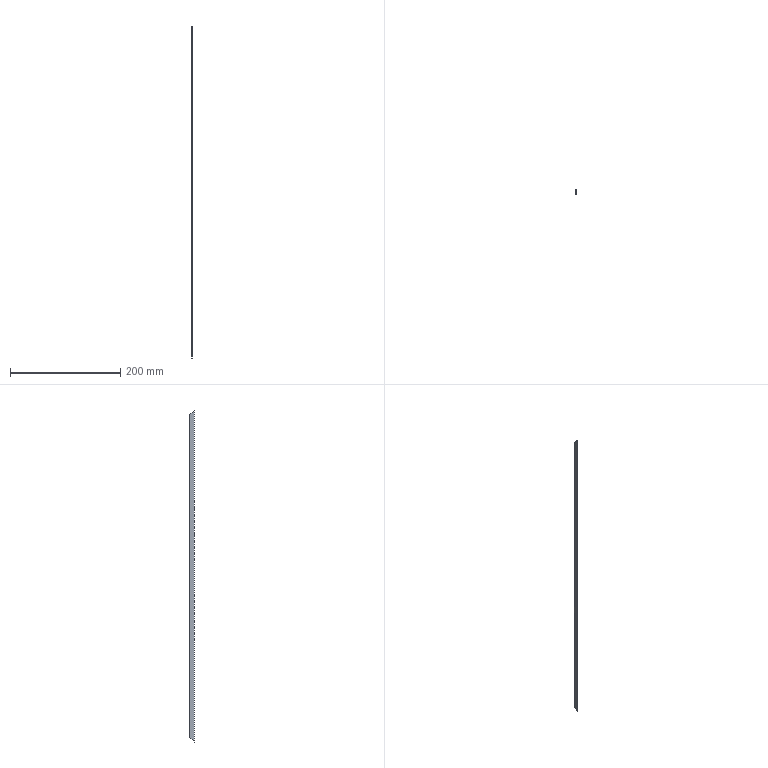Part | NX | features BREP 1 | 1 solid | 6 faces | box 1.5 x 8 x 603 mm | volume 7140 mm3 | plane 6
STEP:
#1=CARTESIAN_POINT('',(0.,8.,293.5));
#2=VERTEX_POINT('',#1);
#3=CARTESIAN_POINT('',(0.,8.,-293.5));
#4=VERTEX_POINT('',#3);
#5=CARTESIAN_POINT('',(0.,8.,301.5));
#6=DIRECTION('',(0.,0.,-1.));
#7=VECTOR('',#6,1000.);
#8=LINE('',#5,#7);
#9=EDGE_CURVE('',#2,#4,#8,.T.);
#10=ORIENTED_EDGE('',*,*,#9,.T.);
#11=CARTESIAN_POINT('',(0.,0.,-301.5));
#12=VERTEX_POINT('',#11);
#13=CARTESIAN_POINT('',(0.,8.,-293.5));
#14=DIRECTION('',(0.,-0.7071,-0.7071));
#15=VECTOR('',#14,1000.);
#16=LINE('',#13,#15);
#17=EDGE_CURVE('',#4,#12,#16,.T.);
#18=ORIENTED_EDGE('',*,*,#17,.T.);
#19=CARTESIAN_POINT('',(0.,0.,301.5));
#20=VERTEX_POINT('',#19);
#21=CARTESIAN_POINT('',(0.,0.,301.5));
#22=DIRECTION('',(0.,0.,-1.));
#23=VECTOR('',#22,1000.);
#24=LINE('',#21,#23);
#25=EDGE_CURVE('',#20,#12,#24,.T.);
#26=ORIENTED_EDGE('',*,*,#25,.F.);
#27=CARTESIAN_POINT('',(0.,0.,301.5));
#28=DIRECTION('',(0.,0.7071,-0.7071));
#29=VECTOR('',#28,1000.);
#30=LINE('',#27,#29);
#31=EDGE_CURVE('',#20,#2,#30,.T.);
#32=ORIENTED_EDGE('',*,*,#31,.T.);
#33=EDGE_LOOP('',(#10,#18,#26,#32));
#34=FACE_BOUND('',#33,.T.);
#35=CARTESIAN_POINT('',(0.,0.,301.5));
#36=DIRECTION('',(1.,0.,0.));
#37=DIRECTION('',(0.,1.,0.));
#38=AXIS2_PLACEMENT_3D('',#35,#36,#37);
#39=PLANE('',#38);
#40=ADVANCED_FACE('',(#34),#39,.F.);
#41=CARTESIAN_POINT('',(1.5,0.,-301.5));
#42=VERTEX_POINT('',#41);
#43=CARTESIAN_POINT('',(0.,0.,-301.5));
#44=DIRECTION('',(1.,0.,0.));
#45=VECTOR('',#44,1000.);
#46=LINE('',#43,#45);
#47=EDGE_CURVE('',#12,#42,#46,.T.);
#48=ORIENTED_EDGE('',*,*,#47,.T.);
#49=CARTESIAN_POINT('',(1.5,0.,301.5));
#50=VERTEX_POINT('',#49);
#51=CARTESIAN_POINT('',(1.5,0.,301.5));
#52=DIRECTION('',(0.,0.,-1.));
#53=VECTOR('',#52,1000.);
#54=LINE('',#51,#53);
#55=EDGE_CURVE('',#50,#42,#54,.T.);
#56=ORIENTED_EDGE('',*,*,#55,.F.);
#57=CARTESIAN_POINT('',(0.,0.,301.5));
#58=DIRECTION('',(1.,0.,0.));
#59=VECTOR('',#58,1000.);
#60=LINE('',#57,#59);
#61=EDGE_CURVE('',#20,#50,#60,.T.);
#62=ORIENTED_EDGE('',*,*,#61,.F.);
#63=ORIENTED_EDGE('',*,*,#25,.T.);
#64=EDGE_LOOP('',(#48,#56,#62,#63));
#65=FACE_BOUND('',#64,.T.);
#66=CARTESIAN_POINT('',(0.,0.,301.5));
#67=DIRECTION('',(0.,1.,0.));
#68=DIRECTION('',(1.,0.,0.));
#69=AXIS2_PLACEMENT_3D('',#66,#67,#68);
#70=PLANE('',#69);
#71=ADVANCED_FACE('',(#65),#70,.F.);
#72=ORIENTED_EDGE('',*,*,#55,.T.);
#73=CARTESIAN_POINT('',(1.5,8.,-293.5));
#74=VERTEX_POINT('',#73);
#75=CARTESIAN_POINT('',(1.5,8.,-293.5));
#76=DIRECTION('',(0.,0.7071,0.7071));
#77=VECTOR('',#76,1000.);
#78=LINE('',#75,#77);
#79=EDGE_CURVE('',#42,#74,#78,.T.);
#80=ORIENTED_EDGE('',*,*,#79,.T.);
#81=CARTESIAN_POINT('',(1.5,8.,293.5));
#82=VERTEX_POINT('',#81);
#83=CARTESIAN_POINT('',(1.5,8.,301.5));
#84=DIRECTION('',(0.,0.,-1.));
#85=VECTOR('',#84,1000.);
#86=LINE('',#83,#85);
#87=EDGE_CURVE('',#82,#74,#86,.T.);
#88=ORIENTED_EDGE('',*,*,#87,.F.);
#89=CARTESIAN_POINT('',(1.5,0.,301.5));
#90=DIRECTION('',(0.,-0.7071,0.7071));
#91=VECTOR('',#90,1000.);
#92=LINE('',#89,#91);
#93=EDGE_CURVE('',#82,#50,#92,.T.);
#94=ORIENTED_EDGE('',*,*,#93,.T.);
#95=EDGE_LOOP('',(#72,#80,#88,#94));
#96=FACE_BOUND('',#95,.T.);
#97=CARTESIAN_POINT('',(1.5,0.,301.5));
#98=DIRECTION('',(-1.,0.,0.));
#99=DIRECTION('',(0.,0.,1.));
#100=AXIS2_PLACEMENT_3D('',#97,#98,#99);
#101=PLANE('',#100);
#102=ADVANCED_FACE('',(#96),#101,.F.);
#103=ORIENTED_EDGE('',*,*,#87,.T.);
#104=CARTESIAN_POINT('',(0.,8.,-293.5));
#105=DIRECTION('',(-1.,0.,0.));
#106=VECTOR('',#105,1000.);
#107=LINE('',#104,#106);
#108=EDGE_CURVE('',#74,#4,#107,.T.);
#109=ORIENTED_EDGE('',*,*,#108,.T.);
#110=ORIENTED_EDGE('',*,*,#9,.F.);
#111=CARTESIAN_POINT('',(0.,8.,293.5));
#112=DIRECTION('',(1.,0.,0.));
#113=VECTOR('',#112,1000.);
#114=LINE('',#111,#113);
#115=EDGE_CURVE('',#2,#82,#114,.T.);
#116=ORIENTED_EDGE('',*,*,#115,.T.);
#117=EDGE_LOOP('',(#103,#109,#110,#116));
#118=FACE_BOUND('',#117,.T.);
#119=CARTESIAN_POINT('',(0.,8.,301.5));
#120=DIRECTION('',(0.,-1.,0.));
#121=DIRECTION('',(0.,0.,-1.));
#122=AXIS2_PLACEMENT_3D('',#119,#120,#121);
#123=PLANE('',#122);
#124=ADVANCED_FACE('',(#118),#123,.F.);
#125=ORIENTED_EDGE('',*,*,#79,.F.);
#126=ORIENTED_EDGE('',*,*,#47,.F.);
#127=ORIENTED_EDGE('',*,*,#17,.F.);
#128=ORIENTED_EDGE('',*,*,#108,.F.);
#129=EDGE_LOOP('',(#125,#126,#127,#128));
#130=FACE_BOUND('',#129,.T.);
#131=CARTESIAN_POINT('',(0.,8.,-293.5));
#132=DIRECTION('',(0.,0.7071,-0.7071));
#133=DIRECTION('',(-1.,0.,0.));
#134=AXIS2_PLACEMENT_3D('',#131,#132,#133);
#135=PLANE('',#134);
#136=ADVANCED_FACE('',(#130),#135,.T.);
#137=ORIENTED_EDGE('',*,*,#93,.F.);
#138=ORIENTED_EDGE('',*,*,#115,.F.);
#139=ORIENTED_EDGE('',*,*,#31,.F.);
#140=ORIENTED_EDGE('',*,*,#61,.T.);
#141=EDGE_LOOP('',(#137,#138,#139,#140));
#142=FACE_BOUND('',#141,.T.);
#143=CARTESIAN_POINT('',(0.,0.,301.5));
#144=DIRECTION('',(0.,-0.7071,-0.7071));
#145=DIRECTION('',(0.,0.7071,-0.7071));
#146=AXIS2_PLACEMENT_3D('',#143,#144,#145);
#147=PLANE('',#146);
#148=ADVANCED_FACE('',(#142),#147,.F.);
#149=CLOSED_SHELL('',(#40,#71,#102,#124,#136,#148));
#150=MANIFOLD_SOLID_BREP('',#149);
#151=(LENGTH_UNIT()NAMED_UNIT(*)SI_UNIT(.MILLI.,.METRE.));
#152=UNCERTAINTY_MEASURE_WITH_UNIT(LENGTH_MEASURE(0.00001),#151,'','');
#153=(NAMED_UNIT(*)PLANE_ANGLE_UNIT()SI_UNIT($,.RADIAN.));
#154=(NAMED_UNIT(*)SI_UNIT($,.STERADIAN.)SOLID_ANGLE_UNIT());
#155=(GEOMETRIC_REPRESENTATION_CONTEXT(3)GLOBAL_UNCERTAINTY_ASSIGNED_CONTEXT((#152))GLOBAL_UNIT_ASSIGNED_CONTEXT((#151,#153,#154))REPRESENTATION_CONTEXT('',''));
#156=ADVANCED_BREP_SHAPE_REPRESENTATION('',(#150),#155);